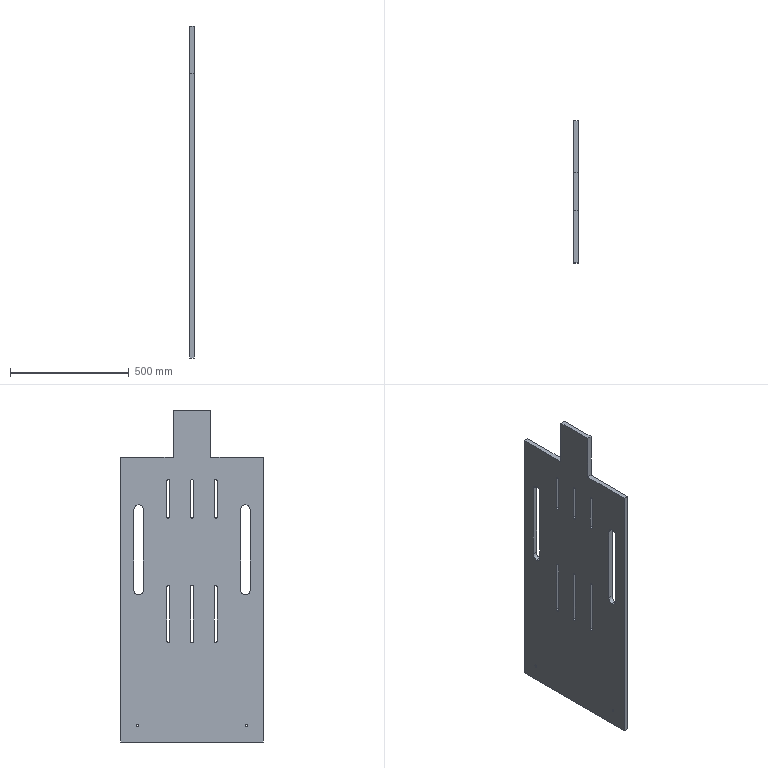Part | STEP file | B1-002 | 1 solid | 63 faces | box 20.1 x 600 x 1400 mm | volume 14156369 mm3 | plane 35 | cylinder 28 | commonest cylinder face diameters 12 x18 40 x6 10.5 x4